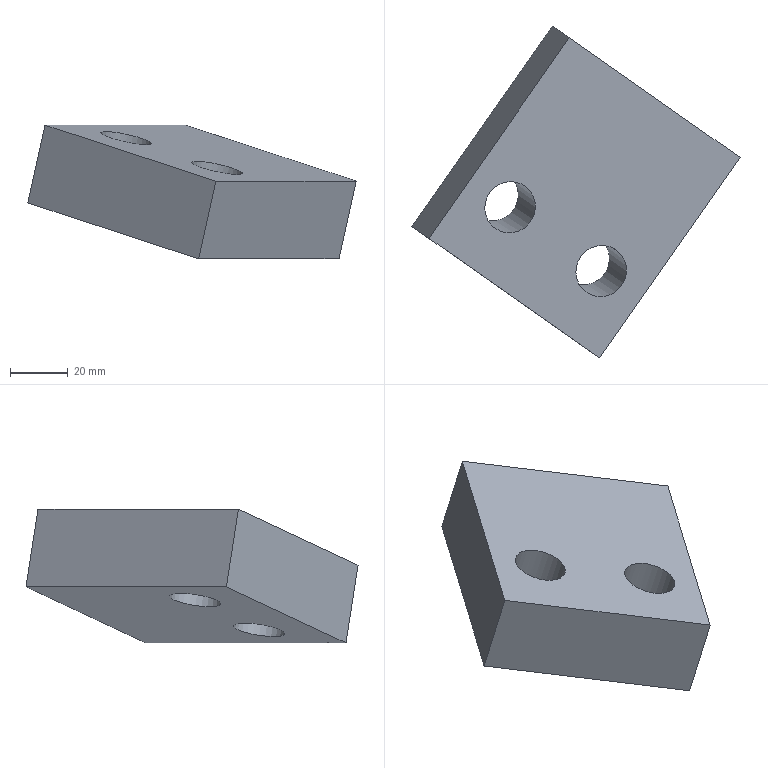Part | NX | features solid 2 | 1 solid | 8 faces | box 114.033 x 115.337 x 46.457 mm | volume 164250 mm3 | plane 6 | cylinder 2 | commonest cylinder face diameters 18 x2
STEP:
#1=CARTESIAN_POINT('',(-725.145,239.867,2.682));
#2=VERTEX_POINT('',#1);
#3=CARTESIAN_POINT('',(-733.936,239.867,4.611));
#4=DIRECTION('',(0.212,-0.1485,0.9659));
#5=DIRECTION('',(0.9767,0.,-0.2144));
#6=AXIS2_PLACEMENT_3D('',#3,#4,#5);
#7=CIRCLE('',#6,9.);
#8=EDGE_CURVE('',#2,#2,#7,.F.);
#9=ORIENTED_EDGE('',*,*,#8,.F.);
#10=EDGE_LOOP('',(#9));
#11=FACE_BOUND('',#10,.T.);
#12=CARTESIAN_POINT('',(-693.495,217.706,-7.671));
#13=VERTEX_POINT('',#12);
#14=CARTESIAN_POINT('',(-702.286,217.706,-5.741));
#15=DIRECTION('',(0.212,-0.1485,0.9659));
#16=DIRECTION('',(0.9767,0.,-0.2144));
#17=AXIS2_PLACEMENT_3D('',#14,#15,#16);
#18=CIRCLE('',#17,9.);
#19=EDGE_CURVE('',#13,#13,#18,.F.);
#20=ORIENTED_EDGE('',*,*,#19,.F.);
#21=EDGE_LOOP('',(#20));
#22=FACE_BOUND('',#21,.T.);
#23=CARTESIAN_POINT('',(-702.779,187.532,-10.271));
#24=VERTEX_POINT('',#23);
#25=CARTESIAN_POINT('',(-654.025,257.16,-10.271));
#26=VERTEX_POINT('',#25);
#27=CARTESIAN_POINT('',(-413.123,601.203,-10.271));
#28=DIRECTION('',(0.5736,0.8192,0.));
#29=VECTOR('',#28,1000.);
#30=LINE('',#27,#29);
#31=EDGE_CURVE('',#24,#26,#30,.T.);
#32=ORIENTED_EDGE('',*,*,#31,.F.);
#33=CARTESIAN_POINT('',(-762.122,229.084,9.141));
#34=VERTEX_POINT('',#33);
#35=CARTESIAN_POINT('',(-730.472,206.923,-1.212));
#36=DIRECTION('',(-0.7912,0.554,0.2588));
#37=VECTOR('',#36,1000.);
#38=LINE('',#35,#37);
#39=EDGE_CURVE('',#34,#24,#38,.F.);
#40=ORIENTED_EDGE('',*,*,#39,.F.);
#41=CARTESIAN_POINT('',(-713.368,298.712,9.141));
#42=VERTEX_POINT('',#41);
#43=CARTESIAN_POINT('',(-472.466,642.756,9.141));
#44=DIRECTION('',(0.5736,0.8192,0.));
#45=VECTOR('',#44,1000.);
#46=LINE('',#43,#45);
#47=EDGE_CURVE('',#34,#42,#46,.T.);
#48=ORIENTED_EDGE('',*,*,#47,.T.);
#49=CARTESIAN_POINT('',(-681.718,276.551,-1.212));
#50=DIRECTION('',(-0.7912,0.554,0.2588));
#51=VECTOR('',#50,1000.);
#52=LINE('',#49,#51);
#53=EDGE_CURVE('',#42,#26,#52,.F.);
#54=ORIENTED_EDGE('',*,*,#53,.T.);
#55=EDGE_LOOP('',(#32,#40,#48,#54));
#56=FACE_BOUND('',#55,.T.);
#57=CARTESIAN_POINT('',(-480.378,648.296,11.729));
#58=DIRECTION('',(-0.212,0.1485,-0.9659));
#59=DIRECTION('',(-0.1706,0.9676,0.1862));
#60=AXIS2_PLACEMENT_3D('',#57,#58,#59);
#61=PLANE('',#60);
#62=ADVANCED_FACE('',(#11,#22,#56),#61,.T.);
#63=CARTESIAN_POINT('',(-648.088,253.003,16.775));
#64=VERTEX_POINT('',#63);
#65=CARTESIAN_POINT('',(-659.906,261.278,-37.066));
#66=DIRECTION('',(-0.212,0.1485,-0.9659));
#67=VECTOR('',#66,1000.);
#68=LINE('',#65,#67);
#69=EDGE_CURVE('',#26,#64,#68,.F.);
#70=ORIENTED_EDGE('',*,*,#69,.F.);
#71=ORIENTED_EDGE('',*,*,#53,.F.);
#72=CARTESIAN_POINT('',(-707.431,294.555,36.187));
#73=VERTEX_POINT('',#72);
#74=CARTESIAN_POINT('',(-719.249,302.83,-17.655));
#75=DIRECTION('',(-0.212,0.1485,-0.9659));
#76=VECTOR('',#75,1000.);
#77=LINE('',#74,#76);
#78=EDGE_CURVE('',#42,#73,#77,.F.);
#79=ORIENTED_EDGE('',*,*,#78,.T.);
#80=CARTESIAN_POINT('',(-675.782,272.394,25.834));
#81=DIRECTION('',(-0.7912,0.554,0.2588));
#82=VECTOR('',#81,1000.);
#83=LINE('',#80,#82);
#84=EDGE_CURVE('',#73,#64,#83,.F.);
#85=ORIENTED_EDGE('',*,*,#84,.T.);
#86=EDGE_LOOP('',(#70,#71,#79,#85));
#87=FACE_BOUND('',#86,.T.);
#88=CARTESIAN_POINT('',(-687.599,280.669,-28.007));
#89=DIRECTION('',(-0.5736,-0.8192,0.));
#90=DIRECTION('',(-0.8192,0.5736,0.));
#91=AXIS2_PLACEMENT_3D('',#88,#89,#90);
#92=PLANE('',#91);
#93=ADVANCED_FACE('',(#87),#92,.F.);
#94=CARTESIAN_POINT('',(-729.535,244.419,33.333));
#95=VERTEX_POINT('',#94);
#96=CARTESIAN_POINT('',(-727.999,235.711,31.657));
#97=DIRECTION('',(0.212,-0.1485,0.9659));
#98=DIRECTION('',(-0.1706,0.9676,0.1862));
#99=AXIS2_PLACEMENT_3D('',#96,#97,#98);
#100=CIRCLE('',#99,9.);
#101=EDGE_CURVE('',#95,#95,#100,.F.);
#102=ORIENTED_EDGE('',*,*,#101,.T.);
#103=EDGE_LOOP('',(#102));
#104=FACE_BOUND('',#103,.T.);
#105=CARTESIAN_POINT('',(-697.885,222.258,22.98));
#106=VERTEX_POINT('',#105);
#107=CARTESIAN_POINT('',(-696.35,213.549,21.305));
#108=DIRECTION('',(0.212,-0.1485,0.9659));
#109=DIRECTION('',(-0.1706,0.9676,0.1862));
#110=AXIS2_PLACEMENT_3D('',#107,#108,#109);
#111=CIRCLE('',#110,9.);
#112=EDGE_CURVE('',#106,#106,#111,.F.);
#113=ORIENTED_EDGE('',*,*,#112,.T.);
#114=EDGE_LOOP('',(#113));
#115=FACE_BOUND('',#114,.T.);
#116=CARTESIAN_POINT('',(-696.842,183.375,16.775));
#117=VERTEX_POINT('',#116);
#118=CARTESIAN_POINT('',(-407.186,597.047,16.775));
#119=DIRECTION('',(0.5736,0.8192,0.));
#120=VECTOR('',#119,1000.);
#121=LINE('',#118,#120);
#122=EDGE_CURVE('',#117,#64,#121,.T.);
#123=ORIENTED_EDGE('',*,*,#122,.T.);
#124=ORIENTED_EDGE('',*,*,#84,.F.);
#125=CARTESIAN_POINT('',(-756.185,224.927,36.187));
#126=VERTEX_POINT('',#125);
#127=CARTESIAN_POINT('',(-466.529,638.599,36.187));
#128=DIRECTION('',(0.5736,0.8192,0.));
#129=VECTOR('',#128,1000.);
#130=LINE('',#127,#129);
#131=EDGE_CURVE('',#126,#73,#130,.T.);
#132=ORIENTED_EDGE('',*,*,#131,.F.);
#133=CARTESIAN_POINT('',(-724.536,202.766,25.834));
#134=DIRECTION('',(-0.7912,0.554,0.2588));
#135=VECTOR('',#134,1000.);
#136=LINE('',#133,#135);
#137=EDGE_CURVE('',#126,#117,#136,.F.);
#138=ORIENTED_EDGE('',*,*,#137,.T.);
#139=EDGE_LOOP('',(#123,#124,#132,#138));
#140=FACE_BOUND('',#139,.T.);
#141=CARTESIAN_POINT('',(-474.442,644.139,38.775));
#142=DIRECTION('',(-0.212,0.1485,-0.9659));
#143=DIRECTION('',(-0.1706,0.9676,0.1862));
#144=AXIS2_PLACEMENT_3D('',#141,#142,#143);
#145=PLANE('',#144);
#146=ADVANCED_FACE('',(#104,#115,#140),#145,.F.);
#147=CARTESIAN_POINT('',(-708.66,191.65,-37.066));
#148=DIRECTION('',(-0.212,0.1485,-0.9659));
#149=VECTOR('',#148,1000.);
#150=LINE('',#147,#149);
#151=EDGE_CURVE('',#24,#117,#150,.F.);
#152=ORIENTED_EDGE('',*,*,#151,.T.);
#153=ORIENTED_EDGE('',*,*,#137,.F.);
#154=CARTESIAN_POINT('',(-768.003,233.202,-17.655));
#155=DIRECTION('',(-0.212,0.1485,-0.9659));
#156=VECTOR('',#155,1000.);
#157=LINE('',#154,#156);
#158=EDGE_CURVE('',#34,#126,#157,.F.);
#159=ORIENTED_EDGE('',*,*,#158,.F.);
#160=ORIENTED_EDGE('',*,*,#39,.T.);
#161=EDGE_LOOP('',(#152,#153,#159,#160));
#162=FACE_BOUND('',#161,.T.);
#163=CARTESIAN_POINT('',(-736.353,211.041,-28.007));
#164=DIRECTION('',(-0.5736,-0.8192,0.));
#165=DIRECTION('',(-0.8192,0.5736,0.));
#166=AXIS2_PLACEMENT_3D('',#163,#164,#165);
#167=PLANE('',#166);
#168=ADVANCED_FACE('',(#162),#167,.T.);
#169=ORIENTED_EDGE('',*,*,#47,.F.);
#170=ORIENTED_EDGE('',*,*,#158,.T.);
#171=ORIENTED_EDGE('',*,*,#131,.T.);
#172=ORIENTED_EDGE('',*,*,#78,.F.);
#173=EDGE_LOOP('',(#169,#170,#171,#172));
#174=FACE_BOUND('',#173,.T.);
#175=CARTESIAN_POINT('',(-487.73,653.444,-60.406));
#176=DIRECTION('',(-0.7912,0.554,0.2588));
#177=DIRECTION('',(0.5736,0.8192,0.));
#178=AXIS2_PLACEMENT_3D('',#175,#176,#177);
#179=PLANE('',#178);
#180=ADVANCED_FACE('',(#174),#179,.T.);
#181=ORIENTED_EDGE('',*,*,#31,.T.);
#182=ORIENTED_EDGE('',*,*,#69,.T.);
#183=ORIENTED_EDGE('',*,*,#122,.F.);
#184=ORIENTED_EDGE('',*,*,#151,.F.);
#185=EDGE_LOOP('',(#181,#182,#183,#184));
#186=FACE_BOUND('',#185,.T.);
#187=CARTESIAN_POINT('',(-428.387,611.892,-79.817));
#188=DIRECTION('',(-0.7912,0.554,0.2588));
#189=DIRECTION('',(0.5736,0.8192,0.));
#190=AXIS2_PLACEMENT_3D('',#187,#188,#189);
#191=PLANE('',#190);
#192=ADVANCED_FACE('',(#186),#191,.F.);
#193=ORIENTED_EDGE('',*,*,#112,.F.);
#194=EDGE_LOOP('',(#193));
#195=FACE_BOUND('',#194,.T.);
#196=ORIENTED_EDGE('',*,*,#19,.T.);
#197=EDGE_LOOP('',(#196));
#198=FACE_BOUND('',#197,.T.);
#199=CARTESIAN_POINT('',(-701.65,217.261,-2.844));
#200=DIRECTION('',(0.212,-0.1485,0.9659));
#201=DIRECTION('',(0.1706,-0.9676,-0.1862));
#202=AXIS2_PLACEMENT_3D('',#199,#200,#201);
#203=CYLINDRICAL_SURFACE('',#202,9.);
#204=ADVANCED_FACE('',(#195,#198),#203,.F.);
#205=ORIENTED_EDGE('',*,*,#101,.F.);
#206=EDGE_LOOP('',(#205));
#207=FACE_BOUND('',#206,.T.);
#208=ORIENTED_EDGE('',*,*,#8,.T.);
#209=EDGE_LOOP('',(#208));
#210=FACE_BOUND('',#209,.T.);
#211=CARTESIAN_POINT('',(-733.299,239.422,7.509));
#212=DIRECTION('',(0.212,-0.1485,0.9659));
#213=DIRECTION('',(0.1706,-0.9676,-0.1862));
#214=AXIS2_PLACEMENT_3D('',#211,#212,#213);
#215=CYLINDRICAL_SURFACE('',#214,9.);
#216=ADVANCED_FACE('',(#207,#210),#215,.F.);
#217=CLOSED_SHELL('',(#62,#93,#146,#168,#180,#192,#204,#216));
#218=MANIFOLD_SOLID_BREP('',#217);
#219=(LENGTH_UNIT()NAMED_UNIT(*)SI_UNIT(.MILLI.,.METRE.));
#220=UNCERTAINTY_MEASURE_WITH_UNIT(LENGTH_MEASURE(0.00001),#219,'','');
#221=(NAMED_UNIT(*)PLANE_ANGLE_UNIT()SI_UNIT($,.RADIAN.));
#222=(NAMED_UNIT(*)SI_UNIT($,.STERADIAN.)SOLID_ANGLE_UNIT());
#223=(GEOMETRIC_REPRESENTATION_CONTEXT(3)GLOBAL_UNCERTAINTY_ASSIGNED_CONTEXT((#220))GLOBAL_UNIT_ASSIGNED_CONTEXT((#219,#221,#222))REPRESENTATION_CONTEXT('',''));
#224=ADVANCED_BREP_SHAPE_REPRESENTATION('',(#218),#223);